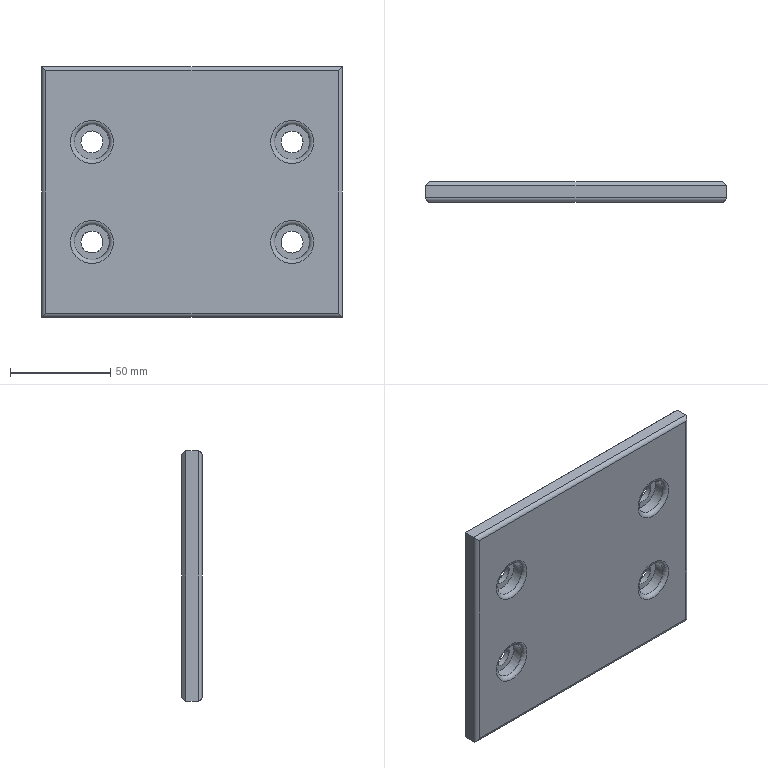Part | NX | features MAIN_BODY 2 | 1 solid | 30 faces | box 150 x 10 x 125 mm | volume 177693 mm3 | plane 14 | cylinder 12 | torus 4 | commonest cylinder face diameters 4 x4 11 x4 17.5 x4
STEP:
#1=CARTESIAN_POINT('',(-298.,285.,-213.));
#2=VERTEX_POINT('',#1);
#3=CARTESIAN_POINT('',(-152.,285.,-213.));
#4=VERTEX_POINT('',#3);
#5=CARTESIAN_POINT('',(-150.,285.,-213.));
#6=DIRECTION('',(-1.,0.,0.));
#7=VECTOR('',#6,1000.);
#8=LINE('',#5,#7);
#9=EDGE_CURVE('',#2,#4,#8,.F.);
#10=ORIENTED_EDGE('',*,*,#9,.T.);
#11=CARTESIAN_POINT('',(-152.,285.,-92.));
#12=VERTEX_POINT('',#11);
#13=CARTESIAN_POINT('',(-152.,285.,-90.));
#14=DIRECTION('',(0.,0.,-1.));
#15=VECTOR('',#14,1000.);
#16=LINE('',#13,#15);
#17=EDGE_CURVE('',#4,#12,#16,.F.);
#18=ORIENTED_EDGE('',*,*,#17,.T.);
#19=CARTESIAN_POINT('',(-298.,285.,-92.));
#20=VERTEX_POINT('',#19);
#21=CARTESIAN_POINT('',(-300.,285.,-92.));
#22=DIRECTION('',(1.,0.,0.));
#23=VECTOR('',#22,1000.);
#24=LINE('',#21,#23);
#25=EDGE_CURVE('',#12,#20,#24,.F.);
#26=ORIENTED_EDGE('',*,*,#25,.T.);
#27=CARTESIAN_POINT('',(-298.,285.,-215.));
#28=DIRECTION('',(0.,0.,1.));
#29=VECTOR('',#28,1000.);
#30=LINE('',#27,#29);
#31=EDGE_CURVE('',#20,#2,#30,.F.);
#32=ORIENTED_EDGE('',*,*,#31,.T.);
#33=EDGE_LOOP('',(#10,#18,#26,#32));
#34=FACE_BOUND('',#33,.T.);
#35=CARTESIAN_POINT('',(-185.75,285.,-177.5));
#36=VERTEX_POINT('',#35);
#37=CARTESIAN_POINT('',(-175.,285.,-177.5));
#38=DIRECTION('',(0.,1.,0.));
#39=DIRECTION('',(-1.,0.,0.));
#40=AXIS2_PLACEMENT_3D('',#37,#38,#39);
#41=CIRCLE('',#40,10.75);
#42=EDGE_CURVE('',#36,#36,#41,.T.);
#43=ORIENTED_EDGE('',*,*,#42,.T.);
#44=EDGE_LOOP('',(#43));
#45=FACE_BOUND('',#44,.T.);
#46=CARTESIAN_POINT('',(-185.75,285.,-127.5));
#47=VERTEX_POINT('',#46);
#48=CARTESIAN_POINT('',(-175.,285.,-127.5));
#49=DIRECTION('',(0.,1.,0.));
#50=DIRECTION('',(-1.,0.,0.));
#51=AXIS2_PLACEMENT_3D('',#48,#49,#50);
#52=CIRCLE('',#51,10.75);
#53=EDGE_CURVE('',#47,#47,#52,.T.);
#54=ORIENTED_EDGE('',*,*,#53,.T.);
#55=EDGE_LOOP('',(#54));
#56=FACE_BOUND('',#55,.T.);
#57=CARTESIAN_POINT('',(-285.75,285.,-127.5));
#58=VERTEX_POINT('',#57);
#59=CARTESIAN_POINT('',(-275.,285.,-127.5));
#60=DIRECTION('',(0.,1.,0.));
#61=DIRECTION('',(-1.,0.,0.));
#62=AXIS2_PLACEMENT_3D('',#59,#60,#61);
#63=CIRCLE('',#62,10.75);
#64=EDGE_CURVE('',#58,#58,#63,.T.);
#65=ORIENTED_EDGE('',*,*,#64,.T.);
#66=EDGE_LOOP('',(#65));
#67=FACE_BOUND('',#66,.T.);
#68=CARTESIAN_POINT('',(-285.75,285.,-177.5));
#69=VERTEX_POINT('',#68);
#70=CARTESIAN_POINT('',(-275.,285.,-177.5));
#71=DIRECTION('',(0.,1.,0.));
#72=DIRECTION('',(-1.,0.,0.));
#73=AXIS2_PLACEMENT_3D('',#70,#71,#72);
#74=CIRCLE('',#73,10.75);
#75=EDGE_CURVE('',#69,#69,#74,.T.);
#76=ORIENTED_EDGE('',*,*,#75,.T.);
#77=EDGE_LOOP('',(#76));
#78=FACE_BOUND('',#77,.T.);
#79=CARTESIAN_POINT('',(-300.,285.,-215.));
#80=DIRECTION('',(0.,1.,0.));
#81=DIRECTION('',(-1.,0.,0.));
#82=AXIS2_PLACEMENT_3D('',#79,#80,#81);
#83=PLANE('',#82);
#84=ADVANCED_FACE('',(#34,#45,#56,#67,#78),#83,.F.);
#85=CARTESIAN_POINT('',(-275.,295.,-133.));
#86=VERTEX_POINT('',#85);
#87=CARTESIAN_POINT('',(-275.,295.,-127.5));
#88=DIRECTION('',(0.,-1.,0.));
#89=DIRECTION('',(0.,0.,-1.));
#90=AXIS2_PLACEMENT_3D('',#87,#88,#89);
#91=CIRCLE('',#90,5.5);
#92=EDGE_CURVE('',#86,#86,#91,.T.);
#93=ORIENTED_EDGE('',*,*,#92,.F.);
#94=EDGE_LOOP('',(#93));
#95=FACE_BOUND('',#94,.T.);
#96=CARTESIAN_POINT('',(-269.5,292.3,-127.5));
#97=VERTEX_POINT('',#96);
#98=CARTESIAN_POINT('',(-275.,292.3,-127.5));
#99=DIRECTION('',(0.,-1.,0.));
#100=DIRECTION('',(1.,0.,0.));
#101=AXIS2_PLACEMENT_3D('',#98,#99,#100);
#102=CIRCLE('',#101,5.5);
#103=EDGE_CURVE('',#97,#97,#102,.T.);
#104=ORIENTED_EDGE('',*,*,#103,.T.);
#105=EDGE_LOOP('',(#104));
#106=FACE_BOUND('',#105,.T.);
#107=CARTESIAN_POINT('',(-275.,275.,-127.5));
#108=DIRECTION('',(0.,1.,0.));
#109=DIRECTION('',(-1.,0.,0.));
#110=AXIS2_PLACEMENT_3D('',#107,#108,#109);
#111=CYLINDRICAL_SURFACE('',#110,5.5);
#112=ADVANCED_FACE('',(#95,#106),#111,.F.);
#113=CARTESIAN_POINT('',(-175.,295.,-172.));
#114=VERTEX_POINT('',#113);
#115=CARTESIAN_POINT('',(-175.,295.,-177.5));
#116=DIRECTION('',(0.,-1.,0.));
#117=DIRECTION('',(0.,0.,1.));
#118=AXIS2_PLACEMENT_3D('',#115,#116,#117);
#119=CIRCLE('',#118,5.5);
#120=EDGE_CURVE('',#114,#114,#119,.T.);
#121=ORIENTED_EDGE('',*,*,#120,.F.);
#122=EDGE_LOOP('',(#121));
#123=FACE_BOUND('',#122,.T.);
#124=CARTESIAN_POINT('',(-169.5,292.3,-177.5));
#125=VERTEX_POINT('',#124);
#126=CARTESIAN_POINT('',(-175.,292.3,-177.5));
#127=DIRECTION('',(0.,-1.,0.));
#128=DIRECTION('',(1.,0.,0.));
#129=AXIS2_PLACEMENT_3D('',#126,#127,#128);
#130=CIRCLE('',#129,5.5);
#131=EDGE_CURVE('',#125,#125,#130,.T.);
#132=ORIENTED_EDGE('',*,*,#131,.T.);
#133=EDGE_LOOP('',(#132));
#134=FACE_BOUND('',#133,.T.);
#135=CARTESIAN_POINT('',(-175.,275.,-177.5));
#136=DIRECTION('',(0.,1.,0.));
#137=DIRECTION('',(-1.,0.,0.));
#138=AXIS2_PLACEMENT_3D('',#135,#136,#137);
#139=CYLINDRICAL_SURFACE('',#138,5.5);
#140=ADVANCED_FACE('',(#123,#134),#139,.F.);
#141=CARTESIAN_POINT('',(-298.,295.,-92.));
#142=VERTEX_POINT('',#141);
#143=CARTESIAN_POINT('',(-152.,295.,-92.));
#144=VERTEX_POINT('',#143);
#145=CARTESIAN_POINT('',(-300.,295.,-92.));
#146=DIRECTION('',(1.,0.,0.));
#147=VECTOR('',#146,1000.);
#148=LINE('',#145,#147);
#149=EDGE_CURVE('',#142,#144,#148,.T.);
#150=ORIENTED_EDGE('',*,*,#149,.T.);
#151=CARTESIAN_POINT('',(-152.,295.,-213.));
#152=VERTEX_POINT('',#151);
#153=CARTESIAN_POINT('',(-152.,295.,-215.));
#154=DIRECTION('',(0.,0.,-1.));
#155=VECTOR('',#154,1000.);
#156=LINE('',#153,#155);
#157=EDGE_CURVE('',#144,#152,#156,.T.);
#158=ORIENTED_EDGE('',*,*,#157,.T.);
#159=CARTESIAN_POINT('',(-298.,295.,-213.));
#160=VERTEX_POINT('',#159);
#161=CARTESIAN_POINT('',(-300.,295.,-213.));
#162=DIRECTION('',(-1.,0.,0.));
#163=VECTOR('',#162,1000.);
#164=LINE('',#161,#163);
#165=EDGE_CURVE('',#152,#160,#164,.T.);
#166=ORIENTED_EDGE('',*,*,#165,.T.);
#167=CARTESIAN_POINT('',(-298.,295.,-215.));
#168=DIRECTION('',(0.,0.,1.));
#169=VECTOR('',#168,1000.);
#170=LINE('',#167,#169);
#171=EDGE_CURVE('',#160,#142,#170,.T.);
#172=ORIENTED_EDGE('',*,*,#171,.T.);
#173=EDGE_LOOP('',(#150,#158,#166,#172));
#174=FACE_BOUND('',#173,.T.);
#175=CARTESIAN_POINT('',(-275.,295.,-172.));
#176=VERTEX_POINT('',#175);
#177=CARTESIAN_POINT('',(-275.,295.,-177.5));
#178=DIRECTION('',(0.,1.,0.));
#179=DIRECTION('',(0.,0.,1.));
#180=AXIS2_PLACEMENT_3D('',#177,#178,#179);
#181=CIRCLE('',#180,5.5);
#182=EDGE_CURVE('',#176,#176,#181,.T.);
#183=ORIENTED_EDGE('',*,*,#182,.F.);
#184=EDGE_LOOP('',(#183));
#185=FACE_BOUND('',#184,.T.);
#186=ORIENTED_EDGE('',*,*,#92,.T.);
#187=EDGE_LOOP('',(#186));
#188=FACE_BOUND('',#187,.T.);
#189=CARTESIAN_POINT('',(-175.,295.,-133.));
#190=VERTEX_POINT('',#189);
#191=CARTESIAN_POINT('',(-175.,295.,-127.5));
#192=DIRECTION('',(0.,1.,0.));
#193=DIRECTION('',(0.,0.,-1.));
#194=AXIS2_PLACEMENT_3D('',#191,#192,#193);
#195=CIRCLE('',#194,5.5);
#196=EDGE_CURVE('',#190,#190,#195,.T.);
#197=ORIENTED_EDGE('',*,*,#196,.F.);
#198=EDGE_LOOP('',(#197));
#199=FACE_BOUND('',#198,.T.);
#200=ORIENTED_EDGE('',*,*,#120,.T.);
#201=EDGE_LOOP('',(#200));
#202=FACE_BOUND('',#201,.T.);
#203=CARTESIAN_POINT('',(-300.,295.,-215.));
#204=DIRECTION('',(0.,1.,0.));
#205=DIRECTION('',(-1.,0.,0.));
#206=AXIS2_PLACEMENT_3D('',#203,#204,#205);
#207=PLANE('',#206);
#208=ADVANCED_FACE('',(#174,#185,#188,#199,#202),#207,.T.);
#209=CARTESIAN_POINT('',(-300.,287.,-215.));
#210=VERTEX_POINT('',#209);
#211=CARTESIAN_POINT('',(-300.,293.,-215.));
#212=VERTEX_POINT('',#211);
#213=CARTESIAN_POINT('',(-300.,285.,-215.));
#214=DIRECTION('',(0.,1.,0.));
#215=VECTOR('',#214,1000.);
#216=LINE('',#213,#215);
#217=EDGE_CURVE('',#210,#212,#216,.T.);
#218=ORIENTED_EDGE('',*,*,#217,.T.);
#219=CARTESIAN_POINT('',(-150.,293.,-215.));
#220=VERTEX_POINT('',#219);
#221=CARTESIAN_POINT('',(-150.,293.,-215.));
#222=DIRECTION('',(1.,0.,0.));
#223=VECTOR('',#222,1000.);
#224=LINE('',#221,#223);
#225=EDGE_CURVE('',#212,#220,#224,.T.);
#226=ORIENTED_EDGE('',*,*,#225,.T.);
#227=CARTESIAN_POINT('',(-150.,287.,-215.));
#228=VERTEX_POINT('',#227);
#229=CARTESIAN_POINT('',(-150.,285.,-215.));
#230=DIRECTION('',(0.,1.,0.));
#231=VECTOR('',#230,1000.);
#232=LINE('',#229,#231);
#233=EDGE_CURVE('',#228,#220,#232,.T.);
#234=ORIENTED_EDGE('',*,*,#233,.F.);
#235=CARTESIAN_POINT('',(-300.,287.,-215.));
#236=DIRECTION('',(-1.,0.,0.));
#237=VECTOR('',#236,1000.);
#238=LINE('',#235,#237);
#239=EDGE_CURVE('',#228,#210,#238,.T.);
#240=ORIENTED_EDGE('',*,*,#239,.T.);
#241=EDGE_LOOP('',(#218,#226,#234,#240));
#242=FACE_BOUND('',#241,.T.);
#243=CARTESIAN_POINT('',(-150.,285.,-215.));
#244=DIRECTION('',(0.,0.,-1.));
#245=DIRECTION('',(1.,0.,0.));
#246=AXIS2_PLACEMENT_3D('',#243,#244,#245);
#247=PLANE('',#246);
#248=ADVANCED_FACE('',(#242),#247,.T.);
#249=CARTESIAN_POINT('',(-300.,287.,-90.));
#250=VERTEX_POINT('',#249);
#251=CARTESIAN_POINT('',(-300.,293.,-90.));
#252=VERTEX_POINT('',#251);
#253=CARTESIAN_POINT('',(-300.,285.,-90.));
#254=DIRECTION('',(0.,1.,0.));
#255=VECTOR('',#254,1000.);
#256=LINE('',#253,#255);
#257=EDGE_CURVE('',#250,#252,#256,.T.);
#258=ORIENTED_EDGE('',*,*,#257,.T.);
#259=CARTESIAN_POINT('',(-300.,293.,-215.));
#260=DIRECTION('',(0.,0.,-1.));
#261=VECTOR('',#260,1000.);
#262=LINE('',#259,#261);
#263=EDGE_CURVE('',#252,#212,#262,.T.);
#264=ORIENTED_EDGE('',*,*,#263,.T.);
#265=ORIENTED_EDGE('',*,*,#217,.F.);
#266=CARTESIAN_POINT('',(-300.,287.,-90.));
#267=DIRECTION('',(0.,0.,1.));
#268=VECTOR('',#267,1000.);
#269=LINE('',#266,#268);
#270=EDGE_CURVE('',#210,#250,#269,.T.);
#271=ORIENTED_EDGE('',*,*,#270,.T.);
#272=EDGE_LOOP('',(#258,#264,#265,#271));
#273=FACE_BOUND('',#272,.T.);
#274=CARTESIAN_POINT('',(-300.,285.,-215.));
#275=DIRECTION('',(-1.,0.,0.));
#276=DIRECTION('',(0.,0.,-1.));
#277=AXIS2_PLACEMENT_3D('',#274,#275,#276);
#278=PLANE('',#277);
#279=ADVANCED_FACE('',(#273),#278,.T.);
#280=CARTESIAN_POINT('',(-150.,287.,-90.));
#281=VERTEX_POINT('',#280);
#282=CARTESIAN_POINT('',(-150.,293.,-90.));
#283=VERTEX_POINT('',#282);
#284=CARTESIAN_POINT('',(-150.,285.,-90.));
#285=DIRECTION('',(0.,1.,0.));
#286=VECTOR('',#285,1000.);
#287=LINE('',#284,#286);
#288=EDGE_CURVE('',#281,#283,#287,.T.);
#289=ORIENTED_EDGE('',*,*,#288,.T.);
#290=CARTESIAN_POINT('',(-300.,293.,-90.));
#291=DIRECTION('',(-1.,0.,0.));
#292=VECTOR('',#291,1000.);
#293=LINE('',#290,#292);
#294=EDGE_CURVE('',#283,#252,#293,.T.);
#295=ORIENTED_EDGE('',*,*,#294,.T.);
#296=ORIENTED_EDGE('',*,*,#257,.F.);
#297=CARTESIAN_POINT('',(-150.,287.,-90.));
#298=DIRECTION('',(1.,0.,0.));
#299=VECTOR('',#298,1000.);
#300=LINE('',#297,#299);
#301=EDGE_CURVE('',#250,#281,#300,.T.);
#302=ORIENTED_EDGE('',*,*,#301,.T.);
#303=EDGE_LOOP('',(#289,#295,#296,#302));
#304=FACE_BOUND('',#303,.T.);
#305=CARTESIAN_POINT('',(-300.,285.,-90.));
#306=DIRECTION('',(0.,0.,1.));
#307=DIRECTION('',(-1.,0.,0.));
#308=AXIS2_PLACEMENT_3D('',#305,#306,#307);
#309=PLANE('',#308);
#310=ADVANCED_FACE('',(#304),#309,.T.);
#311=ORIENTED_EDGE('',*,*,#233,.T.);
#312=CARTESIAN_POINT('',(-150.,293.,-90.));
#313=DIRECTION('',(0.,0.,1.));
#314=VECTOR('',#313,1000.);
#315=LINE('',#312,#314);
#316=EDGE_CURVE('',#220,#283,#315,.T.);
#317=ORIENTED_EDGE('',*,*,#316,.T.);
#318=ORIENTED_EDGE('',*,*,#288,.F.);
#319=CARTESIAN_POINT('',(-150.,287.,-215.));
#320=DIRECTION('',(0.,0.,-1.));
#321=VECTOR('',#320,1000.);
#322=LINE('',#319,#321);
#323=EDGE_CURVE('',#281,#228,#322,.T.);
#324=ORIENTED_EDGE('',*,*,#323,.T.);
#325=EDGE_LOOP('',(#311,#317,#318,#324));
#326=FACE_BOUND('',#325,.T.);
#327=CARTESIAN_POINT('',(-150.,285.,-90.));
#328=DIRECTION('',(1.,0.,0.));
#329=DIRECTION('',(0.,0.,1.));
#330=AXIS2_PLACEMENT_3D('',#327,#328,#329);
#331=PLANE('',#330);
#332=ADVANCED_FACE('',(#326),#331,.T.);
#333=CARTESIAN_POINT('',(-180.5,292.3,-127.5));
#334=VERTEX_POINT('',#333);
#335=CARTESIAN_POINT('',(-175.,292.3,-127.5));
#336=DIRECTION('',(0.,1.,0.));
#337=DIRECTION('',(-1.,0.,0.));
#338=AXIS2_PLACEMENT_3D('',#335,#336,#337);
#339=CIRCLE('',#338,5.5);
#340=EDGE_CURVE('',#334,#334,#339,.F.);
#341=ORIENTED_EDGE('',*,*,#340,.T.);
#342=EDGE_LOOP('',(#341));
#343=FACE_BOUND('',#342,.T.);
#344=ORIENTED_EDGE('',*,*,#196,.T.);
#345=EDGE_LOOP('',(#344));
#346=FACE_BOUND('',#345,.T.);
#347=CARTESIAN_POINT('',(-175.,275.,-127.5));
#348=DIRECTION('',(0.,1.,0.));
#349=DIRECTION('',(-1.,0.,0.));
#350=AXIS2_PLACEMENT_3D('',#347,#348,#349);
#351=CYLINDRICAL_SURFACE('',#350,5.5);
#352=ADVANCED_FACE('',(#343,#346),#351,.F.);
#353=CARTESIAN_POINT('',(-280.5,292.3,-177.5));
#354=VERTEX_POINT('',#353);
#355=CARTESIAN_POINT('',(-275.,292.3,-177.5));
#356=DIRECTION('',(0.,1.,0.));
#357=DIRECTION('',(-1.,0.,0.));
#358=AXIS2_PLACEMENT_3D('',#355,#356,#357);
#359=CIRCLE('',#358,5.5);
#360=EDGE_CURVE('',#354,#354,#359,.F.);
#361=ORIENTED_EDGE('',*,*,#360,.T.);
#362=EDGE_LOOP('',(#361));
#363=FACE_BOUND('',#362,.T.);
#364=ORIENTED_EDGE('',*,*,#182,.T.);
#365=EDGE_LOOP('',(#364));
#366=FACE_BOUND('',#365,.T.);
#367=CARTESIAN_POINT('',(-275.,275.,-177.5));
#368=DIRECTION('',(0.,1.,0.));
#369=DIRECTION('',(-1.,0.,0.));
#370=AXIS2_PLACEMENT_3D('',#367,#368,#369);
#371=CYLINDRICAL_SURFACE('',#370,5.5);
#372=ADVANCED_FACE('',(#363,#366),#371,.F.);
#373=CARTESIAN_POINT('',(-183.75,287.,-177.5));
#374=VERTEX_POINT('',#373);
#375=CARTESIAN_POINT('',(-175.,287.,-177.5));
#376=DIRECTION('',(0.,1.,0.));
#377=DIRECTION('',(-1.,0.,0.));
#378=AXIS2_PLACEMENT_3D('',#375,#376,#377);
#379=CIRCLE('',#378,8.75);
#380=EDGE_CURVE('',#374,#374,#379,.F.);
#381=ORIENTED_EDGE('',*,*,#380,.T.);
#382=EDGE_LOOP('',(#381));
#383=FACE_BOUND('',#382,.T.);
#384=CARTESIAN_POINT('',(-175.,292.3,-168.75));
#385=VERTEX_POINT('',#384);
#386=CARTESIAN_POINT('',(-175.,292.3,-177.5));
#387=DIRECTION('',(0.,-1.,0.));
#388=DIRECTION('',(0.,0.,1.));
#389=AXIS2_PLACEMENT_3D('',#386,#387,#388);
#390=CIRCLE('',#389,8.75);
#391=EDGE_CURVE('',#385,#385,#390,.T.);
#392=ORIENTED_EDGE('',*,*,#391,.F.);
#393=EDGE_LOOP('',(#392));
#394=FACE_BOUND('',#393,.T.);
#395=CARTESIAN_POINT('',(-175.,265.,-177.5));
#396=DIRECTION('',(0.,1.,0.));
#397=DIRECTION('',(-1.,0.,0.));
#398=AXIS2_PLACEMENT_3D('',#395,#396,#397);
#399=CYLINDRICAL_SURFACE('',#398,8.75);
#400=ADVANCED_FACE('',(#383,#394),#399,.F.);
#401=ORIENTED_EDGE('',*,*,#131,.F.);
#402=EDGE_LOOP('',(#401));
#403=FACE_BOUND('',#402,.T.);
#404=ORIENTED_EDGE('',*,*,#391,.T.);
#405=EDGE_LOOP('',(#404));
#406=FACE_BOUND('',#405,.T.);
#407=CARTESIAN_POINT('',(-175.,292.3,-177.5));
#408=DIRECTION('',(0.,-1.,0.));
#409=DIRECTION('',(1.,0.,0.));
#410=AXIS2_PLACEMENT_3D('',#407,#408,#409);
#411=PLANE('',#410);
#412=ADVANCED_FACE('',(#403,#406),#411,.T.);
#413=CARTESIAN_POINT('',(-283.75,287.,-177.5));
#414=VERTEX_POINT('',#413);
#415=CARTESIAN_POINT('',(-275.,287.,-177.5));
#416=DIRECTION('',(0.,1.,0.));
#417=DIRECTION('',(-1.,0.,0.));
#418=AXIS2_PLACEMENT_3D('',#415,#416,#417);
#419=CIRCLE('',#418,8.75);
#420=EDGE_CURVE('',#414,#414,#419,.F.);
#421=ORIENTED_EDGE('',*,*,#420,.T.);
#422=EDGE_LOOP('',(#421));
#423=FACE_BOUND('',#422,.T.);
#424=CARTESIAN_POINT('',(-275.,292.3,-168.75));
#425=VERTEX_POINT('',#424);
#426=CARTESIAN_POINT('',(-275.,292.3,-177.5));
#427=DIRECTION('',(0.,1.,0.));
#428=DIRECTION('',(0.,0.,1.));
#429=AXIS2_PLACEMENT_3D('',#426,#427,#428);
#430=CIRCLE('',#429,8.75);
#431=EDGE_CURVE('',#425,#425,#430,.T.);
#432=ORIENTED_EDGE('',*,*,#431,.T.);
#433=EDGE_LOOP('',(#432));
#434=FACE_BOUND('',#433,.T.);
#435=CARTESIAN_POINT('',(-275.,265.,-177.5));
#436=DIRECTION('',(0.,1.,0.));
#437=DIRECTION('',(-1.,0.,0.));
#438=AXIS2_PLACEMENT_3D('',#435,#436,#437);
#439=CYLINDRICAL_SURFACE('',#438,8.75);
#440=ADVANCED_FACE('',(#423,#434),#439,.F.);
#441=ORIENTED_EDGE('',*,*,#431,.F.);
#442=EDGE_LOOP('',(#441));
#443=FACE_BOUND('',#442,.T.);
#444=ORIENTED_EDGE('',*,*,#360,.F.);
#445=EDGE_LOOP('',(#444));
#446=FACE_BOUND('',#445,.T.);
#447=CARTESIAN_POINT('',(-275.,292.3,-177.5));
#448=DIRECTION('',(0.,1.,0.));
#449=DIRECTION('',(-1.,0.,0.));
#450=AXIS2_PLACEMENT_3D('',#447,#448,#449);
#451=PLANE('',#450);
#452=ADVANCED_FACE('',(#443,#446),#451,.F.);
#453=CARTESIAN_POINT('',(-183.75,287.,-127.5));
#454=VERTEX_POINT('',#453);
#455=CARTESIAN_POINT('',(-175.,287.,-127.5));
#456=DIRECTION('',(0.,1.,0.));
#457=DIRECTION('',(-1.,0.,0.));
#458=AXIS2_PLACEMENT_3D('',#455,#456,#457);
#459=CIRCLE('',#458,8.75);
#460=EDGE_CURVE('',#454,#454,#459,.F.);
#461=ORIENTED_EDGE('',*,*,#460,.T.);
#462=EDGE_LOOP('',(#461));
#463=FACE_BOUND('',#462,.T.);
#464=CARTESIAN_POINT('',(-175.,292.3,-136.25));
#465=VERTEX_POINT('',#464);
#466=CARTESIAN_POINT('',(-175.,292.3,-127.5));
#467=DIRECTION('',(0.,1.,0.));
#468=DIRECTION('',(0.,0.,-1.));
#469=AXIS2_PLACEMENT_3D('',#466,#467,#468);
#470=CIRCLE('',#469,8.75);
#471=EDGE_CURVE('',#465,#465,#470,.T.);
#472=ORIENTED_EDGE('',*,*,#471,.T.);
#473=EDGE_LOOP('',(#472));
#474=FACE_BOUND('',#473,.T.);
#475=CARTESIAN_POINT('',(-175.,265.,-127.5));
#476=DIRECTION('',(0.,1.,0.));
#477=DIRECTION('',(-1.,0.,0.));
#478=AXIS2_PLACEMENT_3D('',#475,#476,#477);
#479=CYLINDRICAL_SURFACE('',#478,8.75);
#480=ADVANCED_FACE('',(#463,#474),#479,.F.);
#481=ORIENTED_EDGE('',*,*,#471,.F.);
#482=EDGE_LOOP('',(#481));
#483=FACE_BOUND('',#482,.T.);
#484=ORIENTED_EDGE('',*,*,#340,.F.);
#485=EDGE_LOOP('',(#484));
#486=FACE_BOUND('',#485,.T.);
#487=CARTESIAN_POINT('',(-175.,292.3,-127.5));
#488=DIRECTION('',(0.,1.,0.));
#489=DIRECTION('',(-1.,0.,0.));
#490=AXIS2_PLACEMENT_3D('',#487,#488,#489);
#491=PLANE('',#490);
#492=ADVANCED_FACE('',(#483,#486),#491,.F.);
#493=CARTESIAN_POINT('',(-283.75,287.,-127.5));
#494=VERTEX_POINT('',#493);
#495=CARTESIAN_POINT('',(-275.,287.,-127.5));
#496=DIRECTION('',(0.,1.,0.));
#497=DIRECTION('',(-1.,0.,0.));
#498=AXIS2_PLACEMENT_3D('',#495,#496,#497);
#499=CIRCLE('',#498,8.75);
#500=EDGE_CURVE('',#494,#494,#499,.F.);
#501=ORIENTED_EDGE('',*,*,#500,.T.);
#502=EDGE_LOOP('',(#501));
#503=FACE_BOUND('',#502,.T.);
#504=CARTESIAN_POINT('',(-275.,292.3,-136.25));
#505=VERTEX_POINT('',#504);
#506=CARTESIAN_POINT('',(-275.,292.3,-127.5));
#507=DIRECTION('',(0.,-1.,0.));
#508=DIRECTION('',(0.,0.,-1.));
#509=AXIS2_PLACEMENT_3D('',#506,#507,#508);
#510=CIRCLE('',#509,8.75);
#511=EDGE_CURVE('',#505,#505,#510,.T.);
#512=ORIENTED_EDGE('',*,*,#511,.F.);
#513=EDGE_LOOP('',(#512));
#514=FACE_BOUND('',#513,.T.);
#515=CARTESIAN_POINT('',(-275.,265.,-127.5));
#516=DIRECTION('',(0.,1.,0.));
#517=DIRECTION('',(-1.,0.,0.));
#518=AXIS2_PLACEMENT_3D('',#515,#516,#517);
#519=CYLINDRICAL_SURFACE('',#518,8.75);
#520=ADVANCED_FACE('',(#503,#514),#519,.F.);
#521=ORIENTED_EDGE('',*,*,#103,.F.);
#522=EDGE_LOOP('',(#521));
#523=FACE_BOUND('',#522,.T.);
#524=ORIENTED_EDGE('',*,*,#511,.T.);
#525=EDGE_LOOP('',(#524));
#526=FACE_BOUND('',#525,.T.);
#527=CARTESIAN_POINT('',(-275.,292.3,-127.5));
#528=DIRECTION('',(0.,-1.,0.));
#529=DIRECTION('',(1.,0.,0.));
#530=AXIS2_PLACEMENT_3D('',#527,#528,#529);
#531=PLANE('',#530);
#532=ADVANCED_FACE('',(#523,#526),#531,.T.);
#533=CARTESIAN_POINT('',(-298.,287.,-213.));
#534=DIRECTION('',(0.7071,0.,-0.7071));
#535=DIRECTION('',(-0.7071,0.,-0.7071));
#536=AXIS2_PLACEMENT_3D('',#533,#534,#535);
#537=ELLIPSE('',#536,2.828,2.);
#538=EDGE_CURVE('',#2,#210,#537,.T.);
#539=ORIENTED_EDGE('',*,*,#538,.F.);
#540=ORIENTED_EDGE('',*,*,#31,.F.);
#541=CARTESIAN_POINT('',(-298.,287.,-92.));
#542=DIRECTION('',(-0.7071,0.,-0.7071));
#543=DIRECTION('',(0.7071,0.,-0.7071));
#544=AXIS2_PLACEMENT_3D('',#541,#542,#543);
#545=ELLIPSE('',#544,2.828,2.);
#546=EDGE_CURVE('',#250,#20,#545,.F.);
#547=ORIENTED_EDGE('',*,*,#546,.F.);
#548=ORIENTED_EDGE('',*,*,#270,.F.);
#549=EDGE_LOOP('',(#539,#540,#547,#548));
#550=FACE_BOUND('',#549,.T.);
#551=CARTESIAN_POINT('',(-298.,287.,-215.));
#552=DIRECTION('',(0.,0.,-1.));
#553=DIRECTION('',(1.,0.,0.));
#554=AXIS2_PLACEMENT_3D('',#551,#552,#553);
#555=CYLINDRICAL_SURFACE('',#554,2.);
#556=ADVANCED_FACE('',(#550),#555,.T.);
#557=ORIENTED_EDGE('',*,*,#546,.T.);
#558=ORIENTED_EDGE('',*,*,#25,.F.);
#559=CARTESIAN_POINT('',(-152.,287.,-92.));
#560=DIRECTION('',(-0.7071,0.,0.7071));
#561=DIRECTION('',(-0.7071,0.,-0.7071));
#562=AXIS2_PLACEMENT_3D('',#559,#560,#561);
#563=ELLIPSE('',#562,2.828,2.);
#564=EDGE_CURVE('',#281,#12,#563,.F.);
#565=ORIENTED_EDGE('',*,*,#564,.F.);
#566=ORIENTED_EDGE('',*,*,#301,.F.);
#567=EDGE_LOOP('',(#557,#558,#565,#566));
#568=FACE_BOUND('',#567,.T.);
#569=CARTESIAN_POINT('',(-300.,287.,-92.));
#570=DIRECTION('',(-1.,0.,0.));
#571=DIRECTION('',(0.,-1.,0.));
#572=AXIS2_PLACEMENT_3D('',#569,#570,#571);
#573=CYLINDRICAL_SURFACE('',#572,2.);
#574=ADVANCED_FACE('',(#568),#573,.T.);
#575=ORIENTED_EDGE('',*,*,#538,.T.);
#576=ORIENTED_EDGE('',*,*,#239,.F.);
#577=CARTESIAN_POINT('',(-152.,287.,-213.));
#578=DIRECTION('',(0.7071,0.,0.7071));
#579=DIRECTION('',(0.7071,0.,-0.7071));
#580=AXIS2_PLACEMENT_3D('',#577,#578,#579);
#581=ELLIPSE('',#580,2.828,2.);
#582=EDGE_CURVE('',#4,#228,#581,.T.);
#583=ORIENTED_EDGE('',*,*,#582,.F.);
#584=ORIENTED_EDGE('',*,*,#9,.F.);
#585=EDGE_LOOP('',(#575,#576,#583,#584));
#586=FACE_BOUND('',#585,.T.);
#587=CARTESIAN_POINT('',(-150.,287.,-213.));
#588=DIRECTION('',(1.,0.,0.));
#589=DIRECTION('',(0.,0.,1.));
#590=AXIS2_PLACEMENT_3D('',#587,#588,#589);
#591=CYLINDRICAL_SURFACE('',#590,2.);
#592=ADVANCED_FACE('',(#586),#591,.T.);
#593=ORIENTED_EDGE('',*,*,#564,.T.);
#594=ORIENTED_EDGE('',*,*,#17,.F.);
#595=ORIENTED_EDGE('',*,*,#582,.T.);
#596=ORIENTED_EDGE('',*,*,#323,.F.);
#597=EDGE_LOOP('',(#593,#594,#595,#596));
#598=FACE_BOUND('',#597,.T.);
#599=CARTESIAN_POINT('',(-152.,287.,-90.));
#600=DIRECTION('',(0.,0.,1.));
#601=DIRECTION('',(-1.,0.,0.));
#602=AXIS2_PLACEMENT_3D('',#599,#600,#601);
#603=CYLINDRICAL_SURFACE('',#602,2.);
#604=ADVANCED_FACE('',(#598),#603,.T.);
#605=ORIENTED_EDGE('',*,*,#42,.F.);
#606=EDGE_LOOP('',(#605));
#607=FACE_BOUND('',#606,.T.);
#608=ORIENTED_EDGE('',*,*,#380,.F.);
#609=EDGE_LOOP('',(#608));
#610=FACE_BOUND('',#609,.T.);
#611=CARTESIAN_POINT('',(-175.,287.,-177.5));
#612=DIRECTION('',(0.,1.,0.));
#613=DIRECTION('',(-1.,0.,0.));
#614=AXIS2_PLACEMENT_3D('',#611,#612,#613);
#615=TOROIDAL_SURFACE('',#614,10.75,2.);
#616=ADVANCED_FACE('',(#607,#610),#615,.T.);
#617=ORIENTED_EDGE('',*,*,#460,.F.);
#618=EDGE_LOOP('',(#617));
#619=FACE_BOUND('',#618,.T.);
#620=ORIENTED_EDGE('',*,*,#53,.F.);
#621=EDGE_LOOP('',(#620));
#622=FACE_BOUND('',#621,.T.);
#623=CARTESIAN_POINT('',(-175.,287.,-127.5));
#624=DIRECTION('',(0.,1.,0.));
#625=DIRECTION('',(-1.,0.,0.));
#626=AXIS2_PLACEMENT_3D('',#623,#624,#625);
#627=TOROIDAL_SURFACE('',#626,10.75,2.);
#628=ADVANCED_FACE('',(#619,#622),#627,.T.);
#629=ORIENTED_EDGE('',*,*,#64,.F.);
#630=EDGE_LOOP('',(#629));
#631=FACE_BOUND('',#630,.T.);
#632=ORIENTED_EDGE('',*,*,#500,.F.);
#633=EDGE_LOOP('',(#632));
#634=FACE_BOUND('',#633,.T.);
#635=CARTESIAN_POINT('',(-275.,287.,-127.5));
#636=DIRECTION('',(0.,1.,0.));
#637=DIRECTION('',(-1.,0.,0.));
#638=AXIS2_PLACEMENT_3D('',#635,#636,#637);
#639=TOROIDAL_SURFACE('',#638,10.75,2.);
#640=ADVANCED_FACE('',(#631,#634),#639,.T.);
#641=ORIENTED_EDGE('',*,*,#420,.F.);
#642=EDGE_LOOP('',(#641));
#643=FACE_BOUND('',#642,.T.);
#644=ORIENTED_EDGE('',*,*,#75,.F.);
#645=EDGE_LOOP('',(#644));
#646=FACE_BOUND('',#645,.T.);
#647=CARTESIAN_POINT('',(-275.,287.,-177.5));
#648=DIRECTION('',(0.,1.,0.));
#649=DIRECTION('',(-1.,0.,0.));
#650=AXIS2_PLACEMENT_3D('',#647,#648,#649);
#651=TOROIDAL_SURFACE('',#650,10.75,2.);
#652=ADVANCED_FACE('',(#643,#646),#651,.T.);
#653=CARTESIAN_POINT('',(-298.667,294.333,-213.667));
#654=DIRECTION('',(-0.5774,-0.5774,-0.5774));
#655=VECTOR('',#654,1000.);
#656=LINE('',#653,#655);
#657=EDGE_CURVE('',#212,#160,#656,.F.);
#658=ORIENTED_EDGE('',*,*,#657,.F.);
#659=ORIENTED_EDGE('',*,*,#263,.F.);
#660=CARTESIAN_POINT('',(-298.667,294.333,-91.333));
#661=DIRECTION('',(-0.5774,-0.5774,0.5774));
#662=VECTOR('',#661,1000.);
#663=LINE('',#660,#662);
#664=EDGE_CURVE('',#142,#252,#663,.T.);
#665=ORIENTED_EDGE('',*,*,#664,.F.);
#666=ORIENTED_EDGE('',*,*,#171,.F.);
#667=EDGE_LOOP('',(#658,#659,#665,#666));
#668=FACE_BOUND('',#667,.T.);
#669=CARTESIAN_POINT('',(-298.,295.,-215.));
#670=DIRECTION('',(0.7071,-0.7071,0.));
#671=DIRECTION('',(0.7071,0.7071,0.));
#672=AXIS2_PLACEMENT_3D('',#669,#670,#671);
#673=PLANE('',#672);
#674=ADVANCED_FACE('',(#668),#673,.F.);
#675=ORIENTED_EDGE('',*,*,#664,.T.);
#676=ORIENTED_EDGE('',*,*,#294,.F.);
#677=CARTESIAN_POINT('',(-201.333,344.333,-141.333));
#678=DIRECTION('',(-0.5774,0.5774,-0.5774));
#679=VECTOR('',#678,1000.);
#680=LINE('',#677,#679);
#681=EDGE_CURVE('',#144,#283,#680,.F.);
#682=ORIENTED_EDGE('',*,*,#681,.F.);
#683=ORIENTED_EDGE('',*,*,#149,.F.);
#684=EDGE_LOOP('',(#675,#676,#682,#683));
#685=FACE_BOUND('',#684,.T.);
#686=CARTESIAN_POINT('',(-300.,295.,-92.));
#687=DIRECTION('',(0.,-0.7071,-0.7071));
#688=DIRECTION('',(0.,-0.7071,0.7071));
#689=AXIS2_PLACEMENT_3D('',#686,#687,#688);
#690=PLANE('',#689);
#691=ADVANCED_FACE('',(#685),#690,.F.);
#692=ORIENTED_EDGE('',*,*,#657,.T.);
#693=ORIENTED_EDGE('',*,*,#165,.F.);
#694=CARTESIAN_POINT('',(-201.333,344.333,-163.667));
#695=DIRECTION('',(0.5774,-0.5774,-0.5774));
#696=VECTOR('',#695,1000.);
#697=LINE('',#694,#696);
#698=EDGE_CURVE('',#220,#152,#697,.F.);
#699=ORIENTED_EDGE('',*,*,#698,.F.);
#700=ORIENTED_EDGE('',*,*,#225,.F.);
#701=EDGE_LOOP('',(#692,#693,#699,#700));
#702=FACE_BOUND('',#701,.T.);
#703=CARTESIAN_POINT('',(-300.,295.,-213.));
#704=DIRECTION('',(0.,-0.7071,0.7071));
#705=DIRECTION('',(0.,0.7071,0.7071));
#706=AXIS2_PLACEMENT_3D('',#703,#704,#705);
#707=PLANE('',#706);
#708=ADVANCED_FACE('',(#702),#707,.F.);
#709=ORIENTED_EDGE('',*,*,#681,.T.);
#710=ORIENTED_EDGE('',*,*,#316,.F.);
#711=ORIENTED_EDGE('',*,*,#698,.T.);
#712=ORIENTED_EDGE('',*,*,#157,.F.);
#713=EDGE_LOOP('',(#709,#710,#711,#712));
#714=FACE_BOUND('',#713,.T.);
#715=CARTESIAN_POINT('',(-152.,295.,-215.));
#716=DIRECTION('',(-0.7071,-0.7071,0.));
#717=DIRECTION('',(0.7071,-0.7071,0.));
#718=AXIS2_PLACEMENT_3D('',#715,#716,#717);
#719=PLANE('',#718);
#720=ADVANCED_FACE('',(#714),#719,.F.);
#721=CLOSED_SHELL('',(#84,#112,#140,#208,#248,#279,#310,#332,#352,#372,#400,#412,#440,#452,#480,#492,#520,#532,#556,#574,#592,#604,#616,#628,#640,#652,#674,#691,#708,#720));
#722=MANIFOLD_SOLID_BREP('',#721);
#723=(LENGTH_UNIT()NAMED_UNIT(*)SI_UNIT(.MILLI.,.METRE.));
#724=UNCERTAINTY_MEASURE_WITH_UNIT(LENGTH_MEASURE(0.00001),#723,'','');
#725=(NAMED_UNIT(*)PLANE_ANGLE_UNIT()SI_UNIT($,.RADIAN.));
#726=(NAMED_UNIT(*)SI_UNIT($,.STERADIAN.)SOLID_ANGLE_UNIT());
#727=(GEOMETRIC_REPRESENTATION_CONTEXT(3)GLOBAL_UNCERTAINTY_ASSIGNED_CONTEXT((#724))GLOBAL_UNIT_ASSIGNED_CONTEXT((#723,#725,#726))REPRESENTATION_CONTEXT('',''));
#728=ADVANCED_BREP_SHAPE_REPRESENTATION('',(#722),#727);